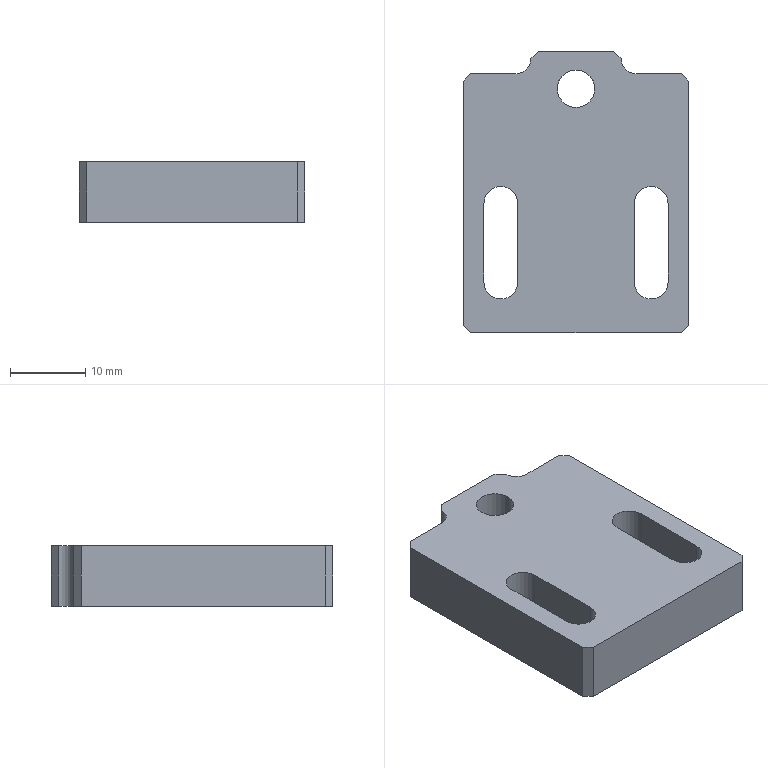Part | NX | features BREP 1 | 1 solid | 26 faces | box 30 x 37.5 x 8 mm | volume 7390 mm3 | plane 18 | cylinder 8 | commonest cylinder face diameters 4.5 x4 4 x2 5 x2
STEP:
#1=CARTESIAN_POINT('',(-6.,17.75,8.));
#2=VERTEX_POINT('',#1);
#3=CARTESIAN_POINT('',(-8.,15.75,8.));
#4=VERTEX_POINT('',#3);
#5=CARTESIAN_POINT('',(-8.,17.75,8.));
#6=DIRECTION('',(0.,0.,-1.));
#7=DIRECTION('',(-1.,0.,0.));
#8=AXIS2_PLACEMENT_3D('',#5,#6,#7);
#9=CIRCLE('',#8,2.);
#10=EDGE_CURVE('',#2,#4,#9,.T.);
#11=ORIENTED_EDGE('',*,*,#10,.F.);
#12=CARTESIAN_POINT('',(-6.,17.75,0.));
#13=VERTEX_POINT('',#12);
#14=CARTESIAN_POINT('',(-6.,17.75,8.));
#15=DIRECTION('',(0.,0.,-1.));
#16=VECTOR('',#15,1000.);
#17=LINE('',#14,#16);
#18=EDGE_CURVE('',#2,#13,#17,.T.);
#19=ORIENTED_EDGE('',*,*,#18,.T.);
#20=CARTESIAN_POINT('',(-8.,15.75,0.));
#21=VERTEX_POINT('',#20);
#22=CARTESIAN_POINT('',(-8.,17.75,0.));
#23=DIRECTION('',(0.,0.,1.));
#24=DIRECTION('',(-1.,0.,0.));
#25=AXIS2_PLACEMENT_3D('',#22,#23,#24);
#26=CIRCLE('',#25,2.);
#27=EDGE_CURVE('',#21,#13,#26,.T.);
#28=ORIENTED_EDGE('',*,*,#27,.F.);
#29=CARTESIAN_POINT('',(-8.,15.75,0.));
#30=DIRECTION('',(0.,0.,-1.));
#31=VECTOR('',#30,1000.);
#32=LINE('',#29,#31);
#33=EDGE_CURVE('',#4,#21,#32,.T.);
#34=ORIENTED_EDGE('',*,*,#33,.F.);
#35=EDGE_LOOP('',(#11,#19,#28,#34));
#36=FACE_BOUND('',#35,.T.);
#37=CARTESIAN_POINT('',(-8.,17.75,8.));
#38=DIRECTION('',(0.,0.,1.));
#39=DIRECTION('',(1.,0.,0.));
#40=AXIS2_PLACEMENT_3D('',#37,#38,#39);
#41=CYLINDRICAL_SURFACE('',#40,2.);
#42=ADVANCED_FACE('',(#36),#41,.F.);
#43=CARTESIAN_POINT('',(8.,15.75,8.));
#44=VERTEX_POINT('',#43);
#45=CARTESIAN_POINT('',(6.,17.75,8.));
#46=VERTEX_POINT('',#45);
#47=CARTESIAN_POINT('',(8.,17.75,8.));
#48=DIRECTION('',(0.,0.,-1.));
#49=DIRECTION('',(-1.,0.,0.));
#50=AXIS2_PLACEMENT_3D('',#47,#48,#49);
#51=CIRCLE('',#50,2.);
#52=EDGE_CURVE('',#44,#46,#51,.T.);
#53=ORIENTED_EDGE('',*,*,#52,.F.);
#54=CARTESIAN_POINT('',(8.,15.75,0.));
#55=VERTEX_POINT('',#54);
#56=CARTESIAN_POINT('',(8.,15.75,8.));
#57=DIRECTION('',(0.,0.,1.));
#58=VECTOR('',#57,1000.);
#59=LINE('',#56,#58);
#60=EDGE_CURVE('',#55,#44,#59,.T.);
#61=ORIENTED_EDGE('',*,*,#60,.F.);
#62=CARTESIAN_POINT('',(6.,17.75,0.));
#63=VERTEX_POINT('',#62);
#64=CARTESIAN_POINT('',(8.,17.75,0.));
#65=DIRECTION('',(0.,0.,1.));
#66=DIRECTION('',(-1.,0.,0.));
#67=AXIS2_PLACEMENT_3D('',#64,#65,#66);
#68=CIRCLE('',#67,2.);
#69=EDGE_CURVE('',#63,#55,#68,.T.);
#70=ORIENTED_EDGE('',*,*,#69,.F.);
#71=CARTESIAN_POINT('',(6.,17.75,8.));
#72=DIRECTION('',(0.,0.,1.));
#73=VECTOR('',#72,1000.);
#74=LINE('',#71,#73);
#75=EDGE_CURVE('',#63,#46,#74,.T.);
#76=ORIENTED_EDGE('',*,*,#75,.T.);
#77=EDGE_LOOP('',(#53,#61,#70,#76));
#78=FACE_BOUND('',#77,.T.);
#79=CARTESIAN_POINT('',(8.,17.75,8.));
#80=DIRECTION('',(0.,0.,1.));
#81=DIRECTION('',(1.,0.,0.));
#82=AXIS2_PLACEMENT_3D('',#79,#80,#81);
#83=CYLINDRICAL_SURFACE('',#82,2.);
#84=ADVANCED_FACE('',(#78),#83,.F.);
#85=CARTESIAN_POINT('',(-5.,18.75,8.));
#86=VERTEX_POINT('',#85);
#87=CARTESIAN_POINT('',(-6.,17.75,8.));
#88=DIRECTION('',(-0.7071,-0.7071,0.));
#89=VECTOR('',#88,1000.);
#90=LINE('',#87,#89);
#91=EDGE_CURVE('',#86,#2,#90,.T.);
#92=ORIENTED_EDGE('',*,*,#91,.F.);
#93=CARTESIAN_POINT('',(-5.,18.75,0.));
#94=VERTEX_POINT('',#93);
#95=CARTESIAN_POINT('',(-5.,18.75,8.));
#96=DIRECTION('',(0.,0.,1.));
#97=VECTOR('',#96,1000.);
#98=LINE('',#95,#97);
#99=EDGE_CURVE('',#94,#86,#98,.T.);
#100=ORIENTED_EDGE('',*,*,#99,.F.);
#101=CARTESIAN_POINT('',(-11.875,11.875,0.));
#102=DIRECTION('',(0.7071,0.7071,0.));
#103=VECTOR('',#102,1000.);
#104=LINE('',#101,#103);
#105=EDGE_CURVE('',#13,#94,#104,.T.);
#106=ORIENTED_EDGE('',*,*,#105,.F.);
#107=ORIENTED_EDGE('',*,*,#18,.F.);
#108=EDGE_LOOP('',(#92,#100,#106,#107));
#109=FACE_BOUND('',#108,.T.);
#110=CARTESIAN_POINT('',(-6.,17.75,8.));
#111=DIRECTION('',(0.7071,-0.7071,0.));
#112=DIRECTION('',(0.,0.,-1.));
#113=AXIS2_PLACEMENT_3D('',#110,#111,#112);
#114=PLANE('',#113);
#115=ADVANCED_FACE('',(#109),#114,.F.);
#116=CARTESIAN_POINT('',(-15.,-17.75,8.));
#117=VERTEX_POINT('',#116);
#118=CARTESIAN_POINT('',(-14.,-18.75,8.));
#119=VERTEX_POINT('',#118);
#120=CARTESIAN_POINT('',(-14.,-18.75,8.));
#121=DIRECTION('',(0.7071,-0.7071,0.));
#122=VECTOR('',#121,1000.);
#123=LINE('',#120,#122);
#124=EDGE_CURVE('',#117,#119,#123,.T.);
#125=ORIENTED_EDGE('',*,*,#124,.F.);
#126=CARTESIAN_POINT('',(-15.,-17.75,0.));
#127=VERTEX_POINT('',#126);
#128=CARTESIAN_POINT('',(-15.,-17.75,8.));
#129=DIRECTION('',(0.,0.,1.));
#130=VECTOR('',#129,1000.);
#131=LINE('',#128,#130);
#132=EDGE_CURVE('',#127,#117,#131,.T.);
#133=ORIENTED_EDGE('',*,*,#132,.F.);
#134=CARTESIAN_POINT('',(-14.,-18.75,0.));
#135=VERTEX_POINT('',#134);
#136=CARTESIAN_POINT('',(-16.375,-16.375,0.));
#137=DIRECTION('',(-0.7071,0.7071,0.));
#138=VECTOR('',#137,1000.);
#139=LINE('',#136,#138);
#140=EDGE_CURVE('',#135,#127,#139,.T.);
#141=ORIENTED_EDGE('',*,*,#140,.F.);
#142=CARTESIAN_POINT('',(-14.,-18.75,8.));
#143=DIRECTION('',(0.,0.,-1.));
#144=VECTOR('',#143,1000.);
#145=LINE('',#142,#144);
#146=EDGE_CURVE('',#119,#135,#145,.T.);
#147=ORIENTED_EDGE('',*,*,#146,.F.);
#148=EDGE_LOOP('',(#125,#133,#141,#147));
#149=FACE_BOUND('',#148,.T.);
#150=CARTESIAN_POINT('',(-14.,-18.75,8.));
#151=DIRECTION('',(0.7071,0.7071,0.));
#152=DIRECTION('',(0.,0.,-1.));
#153=AXIS2_PLACEMENT_3D('',#150,#151,#152);
#154=PLANE('',#153);
#155=ADVANCED_FACE('',(#149),#154,.F.);
#156=CARTESIAN_POINT('',(14.,-18.75,8.));
#157=VERTEX_POINT('',#156);
#158=CARTESIAN_POINT('',(15.,-17.75,8.));
#159=VERTEX_POINT('',#158);
#160=CARTESIAN_POINT('',(15.,-17.75,8.));
#161=DIRECTION('',(0.7071,0.7071,0.));
#162=VECTOR('',#161,1000.);
#163=LINE('',#160,#162);
#164=EDGE_CURVE('',#157,#159,#163,.T.);
#165=ORIENTED_EDGE('',*,*,#164,.F.);
#166=CARTESIAN_POINT('',(14.,-18.75,0.));
#167=VERTEX_POINT('',#166);
#168=CARTESIAN_POINT('',(14.,-18.75,8.));
#169=DIRECTION('',(0.,0.,1.));
#170=VECTOR('',#169,1000.);
#171=LINE('',#168,#170);
#172=EDGE_CURVE('',#167,#157,#171,.T.);
#173=ORIENTED_EDGE('',*,*,#172,.F.);
#174=CARTESIAN_POINT('',(15.,-17.75,0.));
#175=VERTEX_POINT('',#174);
#176=CARTESIAN_POINT('',(16.375,-16.375,0.));
#177=DIRECTION('',(-0.7071,-0.7071,0.));
#178=VECTOR('',#177,1000.);
#179=LINE('',#176,#178);
#180=EDGE_CURVE('',#175,#167,#179,.T.);
#181=ORIENTED_EDGE('',*,*,#180,.F.);
#182=CARTESIAN_POINT('',(15.,-17.75,8.));
#183=DIRECTION('',(0.,0.,-1.));
#184=VECTOR('',#183,1000.);
#185=LINE('',#182,#184);
#186=EDGE_CURVE('',#159,#175,#185,.T.);
#187=ORIENTED_EDGE('',*,*,#186,.F.);
#188=EDGE_LOOP('',(#165,#173,#181,#187));
#189=FACE_BOUND('',#188,.T.);
#190=CARTESIAN_POINT('',(15.,-17.75,8.));
#191=DIRECTION('',(-0.7071,0.7071,0.));
#192=DIRECTION('',(0.,0.,-1.));
#193=AXIS2_PLACEMENT_3D('',#190,#191,#192);
#194=PLANE('',#193);
#195=ADVANCED_FACE('',(#189),#194,.F.);
#196=CARTESIAN_POINT('',(-14.,15.75,8.));
#197=VERTEX_POINT('',#196);
#198=CARTESIAN_POINT('',(-15.,14.75,8.));
#199=VERTEX_POINT('',#198);
#200=CARTESIAN_POINT('',(-15.,14.75,8.));
#201=DIRECTION('',(-0.7071,-0.7071,0.));
#202=VECTOR('',#201,1000.);
#203=LINE('',#200,#202);
#204=EDGE_CURVE('',#197,#199,#203,.T.);
#205=ORIENTED_EDGE('',*,*,#204,.F.);
#206=CARTESIAN_POINT('',(-14.,15.75,0.));
#207=VERTEX_POINT('',#206);
#208=CARTESIAN_POINT('',(-14.,15.75,8.));
#209=DIRECTION('',(0.,0.,1.));
#210=VECTOR('',#209,1000.);
#211=LINE('',#208,#210);
#212=EDGE_CURVE('',#207,#197,#211,.T.);
#213=ORIENTED_EDGE('',*,*,#212,.F.);
#214=CARTESIAN_POINT('',(-15.,14.75,0.));
#215=VERTEX_POINT('',#214);
#216=CARTESIAN_POINT('',(-14.875,14.875,0.));
#217=DIRECTION('',(0.7071,0.7071,0.));
#218=VECTOR('',#217,1000.);
#219=LINE('',#216,#218);
#220=EDGE_CURVE('',#215,#207,#219,.T.);
#221=ORIENTED_EDGE('',*,*,#220,.F.);
#222=CARTESIAN_POINT('',(-15.,14.75,8.));
#223=DIRECTION('',(0.,0.,-1.));
#224=VECTOR('',#223,1000.);
#225=LINE('',#222,#224);
#226=EDGE_CURVE('',#199,#215,#225,.T.);
#227=ORIENTED_EDGE('',*,*,#226,.F.);
#228=EDGE_LOOP('',(#205,#213,#221,#227));
#229=FACE_BOUND('',#228,.T.);
#230=CARTESIAN_POINT('',(-15.,14.75,8.));
#231=DIRECTION('',(0.7071,-0.7071,0.));
#232=DIRECTION('',(0.,0.,-1.));
#233=AXIS2_PLACEMENT_3D('',#230,#231,#232);
#234=PLANE('',#233);
#235=ADVANCED_FACE('',(#229),#234,.F.);
#236=CARTESIAN_POINT('',(15.,14.75,8.));
#237=VERTEX_POINT('',#236);
#238=CARTESIAN_POINT('',(14.,15.75,8.));
#239=VERTEX_POINT('',#238);
#240=CARTESIAN_POINT('',(14.,15.75,8.));
#241=DIRECTION('',(-0.7071,0.7071,0.));
#242=VECTOR('',#241,1000.);
#243=LINE('',#240,#242);
#244=EDGE_CURVE('',#237,#239,#243,.T.);
#245=ORIENTED_EDGE('',*,*,#244,.F.);
#246=CARTESIAN_POINT('',(15.,14.75,0.));
#247=VERTEX_POINT('',#246);
#248=CARTESIAN_POINT('',(15.,14.75,8.));
#249=DIRECTION('',(0.,0.,1.));
#250=VECTOR('',#249,1000.);
#251=LINE('',#248,#250);
#252=EDGE_CURVE('',#247,#237,#251,.T.);
#253=ORIENTED_EDGE('',*,*,#252,.F.);
#254=CARTESIAN_POINT('',(14.,15.75,0.));
#255=VERTEX_POINT('',#254);
#256=CARTESIAN_POINT('',(14.875,14.875,0.));
#257=DIRECTION('',(0.7071,-0.7071,0.));
#258=VECTOR('',#257,1000.);
#259=LINE('',#256,#258);
#260=EDGE_CURVE('',#255,#247,#259,.T.);
#261=ORIENTED_EDGE('',*,*,#260,.F.);
#262=CARTESIAN_POINT('',(14.,15.75,8.));
#263=DIRECTION('',(0.,0.,-1.));
#264=VECTOR('',#263,1000.);
#265=LINE('',#262,#264);
#266=EDGE_CURVE('',#239,#255,#265,.T.);
#267=ORIENTED_EDGE('',*,*,#266,.F.);
#268=EDGE_LOOP('',(#245,#253,#261,#267));
#269=FACE_BOUND('',#268,.T.);
#270=CARTESIAN_POINT('',(14.,15.75,8.));
#271=DIRECTION('',(-0.7071,-0.7071,0.));
#272=DIRECTION('',(0.,0.,-1.));
#273=AXIS2_PLACEMENT_3D('',#270,#271,#272);
#274=PLANE('',#273);
#275=ADVANCED_FACE('',(#269),#274,.F.);
#276=CARTESIAN_POINT('',(5.,18.75,8.));
#277=VERTEX_POINT('',#276);
#278=CARTESIAN_POINT('',(5.,18.75,8.));
#279=DIRECTION('',(-0.7071,0.7071,0.));
#280=VECTOR('',#279,1000.);
#281=LINE('',#278,#280);
#282=EDGE_CURVE('',#46,#277,#281,.T.);
#283=ORIENTED_EDGE('',*,*,#282,.F.);
#284=ORIENTED_EDGE('',*,*,#75,.F.);
#285=CARTESIAN_POINT('',(5.,18.75,0.));
#286=VERTEX_POINT('',#285);
#287=CARTESIAN_POINT('',(11.875,11.875,0.));
#288=DIRECTION('',(0.7071,-0.7071,0.));
#289=VECTOR('',#288,1000.);
#290=LINE('',#287,#289);
#291=EDGE_CURVE('',#286,#63,#290,.T.);
#292=ORIENTED_EDGE('',*,*,#291,.F.);
#293=CARTESIAN_POINT('',(5.,18.75,8.));
#294=DIRECTION('',(0.,0.,-1.));
#295=VECTOR('',#294,1000.);
#296=LINE('',#293,#295);
#297=EDGE_CURVE('',#277,#286,#296,.T.);
#298=ORIENTED_EDGE('',*,*,#297,.F.);
#299=EDGE_LOOP('',(#283,#284,#292,#298));
#300=FACE_BOUND('',#299,.T.);
#301=CARTESIAN_POINT('',(5.,18.75,8.));
#302=DIRECTION('',(-0.7071,-0.7071,0.));
#303=DIRECTION('',(0.,0.,-1.));
#304=AXIS2_PLACEMENT_3D('',#301,#302,#303);
#305=PLANE('',#304);
#306=ADVANCED_FACE('',(#300),#305,.F.);
#307=CARTESIAN_POINT('',(-12.25,-1.5,0.));
#308=VERTEX_POINT('',#307);
#309=CARTESIAN_POINT('',(-12.25,-1.5,8.));
#310=VERTEX_POINT('',#309);
#311=CARTESIAN_POINT('',(-12.25,-1.5,0.));
#312=DIRECTION('',(0.,0.,1.));
#313=VECTOR('',#312,1000.);
#314=LINE('',#311,#313);
#315=EDGE_CURVE('',#308,#310,#314,.T.);
#316=ORIENTED_EDGE('',*,*,#315,.T.);
#317=CARTESIAN_POINT('',(-12.25,-12.,8.));
#318=VERTEX_POINT('',#317);
#319=CARTESIAN_POINT('',(-12.25,-12.,8.));
#320=DIRECTION('',(0.,1.,0.));
#321=VECTOR('',#320,1000.);
#322=LINE('',#319,#321);
#323=EDGE_CURVE('',#318,#310,#322,.T.);
#324=ORIENTED_EDGE('',*,*,#323,.F.);
#325=CARTESIAN_POINT('',(-12.25,-12.,0.));
#326=VERTEX_POINT('',#325);
#327=CARTESIAN_POINT('',(-12.25,-12.,0.));
#328=DIRECTION('',(0.,0.,-1.));
#329=VECTOR('',#328,1000.);
#330=LINE('',#327,#329);
#331=EDGE_CURVE('',#318,#326,#330,.T.);
#332=ORIENTED_EDGE('',*,*,#331,.T.);
#333=CARTESIAN_POINT('',(-12.25,-12.,0.));
#334=DIRECTION('',(0.,1.,0.));
#335=VECTOR('',#334,1000.);
#336=LINE('',#333,#335);
#337=EDGE_CURVE('',#326,#308,#336,.T.);
#338=ORIENTED_EDGE('',*,*,#337,.T.);
#339=EDGE_LOOP('',(#316,#324,#332,#338));
#340=FACE_BOUND('',#339,.T.);
#341=CARTESIAN_POINT('',(-12.25,-12.,0.));
#342=DIRECTION('',(-1.,0.,0.));
#343=DIRECTION('',(0.,0.,1.));
#344=AXIS2_PLACEMENT_3D('',#341,#342,#343);
#345=PLANE('',#344);
#346=ADVANCED_FACE('',(#340),#345,.F.);
#347=CARTESIAN_POINT('',(-7.75,-1.5,0.));
#348=VERTEX_POINT('',#347);
#349=CARTESIAN_POINT('',(-7.75,-1.5,8.));
#350=VERTEX_POINT('',#349);
#351=CARTESIAN_POINT('',(-7.75,-1.5,8.));
#352=DIRECTION('',(0.,0.,1.));
#353=VECTOR('',#352,1000.);
#354=LINE('',#351,#353);
#355=EDGE_CURVE('',#348,#350,#354,.T.);
#356=ORIENTED_EDGE('',*,*,#355,.F.);
#357=CARTESIAN_POINT('',(-7.75,-12.,0.));
#358=VERTEX_POINT('',#357);
#359=CARTESIAN_POINT('',(-7.75,-12.,0.));
#360=DIRECTION('',(0.,1.,0.));
#361=VECTOR('',#360,1000.);
#362=LINE('',#359,#361);
#363=EDGE_CURVE('',#358,#348,#362,.T.);
#364=ORIENTED_EDGE('',*,*,#363,.F.);
#365=CARTESIAN_POINT('',(-7.75,-12.,8.));
#366=VERTEX_POINT('',#365);
#367=CARTESIAN_POINT('',(-7.75,-12.,8.));
#368=DIRECTION('',(0.,0.,1.));
#369=VECTOR('',#368,1000.);
#370=LINE('',#367,#369);
#371=EDGE_CURVE('',#358,#366,#370,.T.);
#372=ORIENTED_EDGE('',*,*,#371,.T.);
#373=CARTESIAN_POINT('',(-7.75,-12.,8.));
#374=DIRECTION('',(0.,1.,0.));
#375=VECTOR('',#374,1000.);
#376=LINE('',#373,#375);
#377=EDGE_CURVE('',#366,#350,#376,.T.);
#378=ORIENTED_EDGE('',*,*,#377,.T.);
#379=EDGE_LOOP('',(#356,#364,#372,#378));
#380=FACE_BOUND('',#379,.T.);
#381=CARTESIAN_POINT('',(-7.75,-12.,8.));
#382=DIRECTION('',(-1.,0.,0.));
#383=DIRECTION('',(0.,0.,1.));
#384=AXIS2_PLACEMENT_3D('',#381,#382,#383);
#385=PLANE('',#384);
#386=ADVANCED_FACE('',(#380),#385,.T.);
#387=CARTESIAN_POINT('',(-10.,-12.,8.));
#388=DIRECTION('',(0.,0.,-1.));
#389=DIRECTION('',(-1.,0.,0.));
#390=AXIS2_PLACEMENT_3D('',#387,#388,#389);
#391=CIRCLE('',#390,2.25);
#392=EDGE_CURVE('',#366,#318,#391,.T.);
#393=ORIENTED_EDGE('',*,*,#392,.F.);
#394=ORIENTED_EDGE('',*,*,#371,.F.);
#395=CARTESIAN_POINT('',(-10.,-12.,0.));
#396=DIRECTION('',(0.,0.,-1.));
#397=DIRECTION('',(-1.,0.,0.));
#398=AXIS2_PLACEMENT_3D('',#395,#396,#397);
#399=CIRCLE('',#398,2.25);
#400=EDGE_CURVE('',#358,#326,#399,.T.);
#401=ORIENTED_EDGE('',*,*,#400,.T.);
#402=ORIENTED_EDGE('',*,*,#331,.F.);
#403=EDGE_LOOP('',(#393,#394,#401,#402));
#404=FACE_BOUND('',#403,.T.);
#405=CARTESIAN_POINT('',(-10.,-12.,0.));
#406=DIRECTION('',(0.,0.,-1.));
#407=DIRECTION('',(-1.,0.,0.));
#408=AXIS2_PLACEMENT_3D('',#405,#406,#407);
#409=CYLINDRICAL_SURFACE('',#408,2.25);
#410=ADVANCED_FACE('',(#404),#409,.F.);
#411=CARTESIAN_POINT('',(-10.,-1.5,0.));
#412=DIRECTION('',(0.,0.,-1.));
#413=DIRECTION('',(-1.,0.,0.));
#414=AXIS2_PLACEMENT_3D('',#411,#412,#413);
#415=CIRCLE('',#414,2.25);
#416=EDGE_CURVE('',#308,#348,#415,.T.);
#417=ORIENTED_EDGE('',*,*,#416,.T.);
#418=ORIENTED_EDGE('',*,*,#355,.T.);
#419=CARTESIAN_POINT('',(-10.,-1.5,8.));
#420=DIRECTION('',(0.,0.,-1.));
#421=DIRECTION('',(-1.,0.,0.));
#422=AXIS2_PLACEMENT_3D('',#419,#420,#421);
#423=CIRCLE('',#422,2.25);
#424=EDGE_CURVE('',#310,#350,#423,.T.);
#425=ORIENTED_EDGE('',*,*,#424,.F.);
#426=ORIENTED_EDGE('',*,*,#315,.F.);
#427=EDGE_LOOP('',(#417,#418,#425,#426));
#428=FACE_BOUND('',#427,.T.);
#429=CARTESIAN_POINT('',(-10.,-1.5,0.));
#430=DIRECTION('',(0.,0.,-1.));
#431=DIRECTION('',(-1.,0.,0.));
#432=AXIS2_PLACEMENT_3D('',#429,#430,#431);
#433=CYLINDRICAL_SURFACE('',#432,2.25);
#434=ADVANCED_FACE('',(#428),#433,.F.);
#435=CARTESIAN_POINT('',(7.75,-1.5,0.));
#436=VERTEX_POINT('',#435);
#437=CARTESIAN_POINT('',(7.75,-1.5,8.));
#438=VERTEX_POINT('',#437);
#439=CARTESIAN_POINT('',(7.75,-1.5,0.));
#440=DIRECTION('',(0.,0.,1.));
#441=VECTOR('',#440,1000.);
#442=LINE('',#439,#441);
#443=EDGE_CURVE('',#436,#438,#442,.T.);
#444=ORIENTED_EDGE('',*,*,#443,.T.);
#445=CARTESIAN_POINT('',(7.75,-12.,8.));
#446=VERTEX_POINT('',#445);
#447=CARTESIAN_POINT('',(7.75,-12.,8.));
#448=DIRECTION('',(0.,1.,0.));
#449=VECTOR('',#448,1000.);
#450=LINE('',#447,#449);
#451=EDGE_CURVE('',#446,#438,#450,.T.);
#452=ORIENTED_EDGE('',*,*,#451,.F.);
#453=CARTESIAN_POINT('',(7.75,-12.,0.));
#454=VERTEX_POINT('',#453);
#455=CARTESIAN_POINT('',(7.75,-12.,0.));
#456=DIRECTION('',(0.,0.,-1.));
#457=VECTOR('',#456,1000.);
#458=LINE('',#455,#457);
#459=EDGE_CURVE('',#446,#454,#458,.T.);
#460=ORIENTED_EDGE('',*,*,#459,.T.);
#461=CARTESIAN_POINT('',(7.75,-12.,0.));
#462=DIRECTION('',(0.,1.,0.));
#463=VECTOR('',#462,1000.);
#464=LINE('',#461,#463);
#465=EDGE_CURVE('',#454,#436,#464,.T.);
#466=ORIENTED_EDGE('',*,*,#465,.T.);
#467=EDGE_LOOP('',(#444,#452,#460,#466));
#468=FACE_BOUND('',#467,.T.);
#469=CARTESIAN_POINT('',(7.75,-12.,0.));
#470=DIRECTION('',(-1.,0.,0.));
#471=DIRECTION('',(0.,0.,1.));
#472=AXIS2_PLACEMENT_3D('',#469,#470,#471);
#473=PLANE('',#472);
#474=ADVANCED_FACE('',(#468),#473,.F.);
#475=CARTESIAN_POINT('',(12.25,-1.5,0.));
#476=VERTEX_POINT('',#475);
#477=CARTESIAN_POINT('',(12.25,-1.5,8.));
#478=VERTEX_POINT('',#477);
#479=CARTESIAN_POINT('',(12.25,-1.5,8.));
#480=DIRECTION('',(0.,0.,1.));
#481=VECTOR('',#480,1000.);
#482=LINE('',#479,#481);
#483=EDGE_CURVE('',#476,#478,#482,.T.);
#484=ORIENTED_EDGE('',*,*,#483,.F.);
#485=CARTESIAN_POINT('',(12.25,-12.,0.));
#486=VERTEX_POINT('',#485);
#487=CARTESIAN_POINT('',(12.25,-12.,0.));
#488=DIRECTION('',(0.,1.,0.));
#489=VECTOR('',#488,1000.);
#490=LINE('',#487,#489);
#491=EDGE_CURVE('',#486,#476,#490,.T.);
#492=ORIENTED_EDGE('',*,*,#491,.F.);
#493=CARTESIAN_POINT('',(12.25,-12.,8.));
#494=VERTEX_POINT('',#493);
#495=CARTESIAN_POINT('',(12.25,-12.,8.));
#496=DIRECTION('',(0.,0.,1.));
#497=VECTOR('',#496,1000.);
#498=LINE('',#495,#497);
#499=EDGE_CURVE('',#486,#494,#498,.T.);
#500=ORIENTED_EDGE('',*,*,#499,.T.);
#501=CARTESIAN_POINT('',(12.25,-12.,8.));
#502=DIRECTION('',(0.,1.,0.));
#503=VECTOR('',#502,1000.);
#504=LINE('',#501,#503);
#505=EDGE_CURVE('',#494,#478,#504,.T.);
#506=ORIENTED_EDGE('',*,*,#505,.T.);
#507=EDGE_LOOP('',(#484,#492,#500,#506));
#508=FACE_BOUND('',#507,.T.);
#509=CARTESIAN_POINT('',(12.25,-12.,8.));
#510=DIRECTION('',(-1.,0.,0.));
#511=DIRECTION('',(0.,0.,1.));
#512=AXIS2_PLACEMENT_3D('',#509,#510,#511);
#513=PLANE('',#512);
#514=ADVANCED_FACE('',(#508),#513,.T.);
#515=CARTESIAN_POINT('',(10.,-12.,8.));
#516=DIRECTION('',(0.,0.,-1.));
#517=DIRECTION('',(-1.,0.,0.));
#518=AXIS2_PLACEMENT_3D('',#515,#516,#517);
#519=CIRCLE('',#518,2.25);
#520=EDGE_CURVE('',#494,#446,#519,.T.);
#521=ORIENTED_EDGE('',*,*,#520,.F.);
#522=ORIENTED_EDGE('',*,*,#499,.F.);
#523=CARTESIAN_POINT('',(10.,-12.,0.));
#524=DIRECTION('',(0.,0.,-1.));
#525=DIRECTION('',(-1.,0.,0.));
#526=AXIS2_PLACEMENT_3D('',#523,#524,#525);
#527=CIRCLE('',#526,2.25);
#528=EDGE_CURVE('',#486,#454,#527,.T.);
#529=ORIENTED_EDGE('',*,*,#528,.T.);
#530=ORIENTED_EDGE('',*,*,#459,.F.);
#531=EDGE_LOOP('',(#521,#522,#529,#530));
#532=FACE_BOUND('',#531,.T.);
#533=CARTESIAN_POINT('',(10.,-12.,0.));
#534=DIRECTION('',(0.,0.,-1.));
#535=DIRECTION('',(-1.,0.,0.));
#536=AXIS2_PLACEMENT_3D('',#533,#534,#535);
#537=CYLINDRICAL_SURFACE('',#536,2.25);
#538=ADVANCED_FACE('',(#532),#537,.F.);
#539=CARTESIAN_POINT('',(10.,-1.5,0.));
#540=DIRECTION('',(0.,0.,-1.));
#541=DIRECTION('',(-1.,0.,0.));
#542=AXIS2_PLACEMENT_3D('',#539,#540,#541);
#543=CIRCLE('',#542,2.25);
#544=EDGE_CURVE('',#436,#476,#543,.T.);
#545=ORIENTED_EDGE('',*,*,#544,.T.);
#546=ORIENTED_EDGE('',*,*,#483,.T.);
#547=CARTESIAN_POINT('',(10.,-1.5,8.));
#548=DIRECTION('',(0.,0.,-1.));
#549=DIRECTION('',(-1.,0.,0.));
#550=AXIS2_PLACEMENT_3D('',#547,#548,#549);
#551=CIRCLE('',#550,2.25);
#552=EDGE_CURVE('',#438,#478,#551,.T.);
#553=ORIENTED_EDGE('',*,*,#552,.F.);
#554=ORIENTED_EDGE('',*,*,#443,.F.);
#555=EDGE_LOOP('',(#545,#546,#553,#554));
#556=FACE_BOUND('',#555,.T.);
#557=CARTESIAN_POINT('',(10.,-1.5,0.));
#558=DIRECTION('',(0.,0.,-1.));
#559=DIRECTION('',(-1.,0.,0.));
#560=AXIS2_PLACEMENT_3D('',#557,#558,#559);
#561=CYLINDRICAL_SURFACE('',#560,2.25);
#562=ADVANCED_FACE('',(#556),#561,.F.);
#563=CARTESIAN_POINT('',(-15.,15.75,8.));
#564=DIRECTION('',(-1.,0.,0.));
#565=VECTOR('',#564,1000.);
#566=LINE('',#563,#565);
#567=EDGE_CURVE('',#4,#197,#566,.T.);
#568=ORIENTED_EDGE('',*,*,#567,.F.);
#569=ORIENTED_EDGE('',*,*,#33,.T.);
#570=CARTESIAN_POINT('',(-15.,15.75,0.));
#571=DIRECTION('',(-1.,0.,0.));
#572=VECTOR('',#571,1000.);
#573=LINE('',#570,#572);
#574=EDGE_CURVE('',#21,#207,#573,.T.);
#575=ORIENTED_EDGE('',*,*,#574,.T.);
#576=ORIENTED_EDGE('',*,*,#212,.T.);
#577=EDGE_LOOP('',(#568,#569,#575,#576));
#578=FACE_BOUND('',#577,.T.);
#579=CARTESIAN_POINT('',(-15.,15.75,8.));
#580=DIRECTION('',(0.,-1.,0.));
#581=DIRECTION('',(0.,0.,-1.));
#582=AXIS2_PLACEMENT_3D('',#579,#580,#581);
#583=PLANE('',#582);
#584=ADVANCED_FACE('',(#578),#583,.F.);
#585=CARTESIAN_POINT('',(15.,15.75,0.));
#586=DIRECTION('',(-1.,0.,0.));
#587=VECTOR('',#586,1000.);
#588=LINE('',#585,#587);
#589=EDGE_CURVE('',#255,#55,#588,.T.);
#590=ORIENTED_EDGE('',*,*,#589,.T.);
#591=ORIENTED_EDGE('',*,*,#60,.T.);
#592=CARTESIAN_POINT('',(15.,15.75,8.));
#593=DIRECTION('',(-1.,0.,0.));
#594=VECTOR('',#593,1000.);
#595=LINE('',#592,#594);
#596=EDGE_CURVE('',#239,#44,#595,.T.);
#597=ORIENTED_EDGE('',*,*,#596,.F.);
#598=ORIENTED_EDGE('',*,*,#266,.T.);
#599=EDGE_LOOP('',(#590,#591,#597,#598));
#600=FACE_BOUND('',#599,.T.);
#601=CARTESIAN_POINT('',(15.,15.75,8.));
#602=DIRECTION('',(0.,-1.,0.));
#603=DIRECTION('',(1.,0.,0.));
#604=AXIS2_PLACEMENT_3D('',#601,#602,#603);
#605=PLANE('',#604);
#606=ADVANCED_FACE('',(#600),#605,.F.);
#607=CARTESIAN_POINT('',(-2.5,13.75,8.));
#608=VERTEX_POINT('',#607);
#609=CARTESIAN_POINT('',(-2.5,13.75,0.));
#610=VERTEX_POINT('',#609);
#611=CARTESIAN_POINT('',(-2.5,13.75,8.));
#612=DIRECTION('',(0.,0.,1.));
#613=VECTOR('',#612,1000.);
#614=LINE('',#611,#613);
#615=EDGE_CURVE('',#608,#610,#614,.F.);
#616=ORIENTED_EDGE('',*,*,#615,.T.);
#617=CARTESIAN_POINT('',(2.5,13.75,0.));
#618=VERTEX_POINT('',#617);
#619=CARTESIAN_POINT('',(0.,13.75,0.));
#620=DIRECTION('',(0.,0.,1.));
#621=DIRECTION('',(1.,0.,0.));
#622=AXIS2_PLACEMENT_3D('',#619,#620,#621);
#623=CIRCLE('',#622,2.5);
#624=EDGE_CURVE('',#618,#610,#623,.T.);
#625=ORIENTED_EDGE('',*,*,#624,.F.);
#626=CARTESIAN_POINT('',(2.5,13.75,8.));
#627=VERTEX_POINT('',#626);
#628=CARTESIAN_POINT('',(2.5,13.75,8.));
#629=DIRECTION('',(0.,0.,1.));
#630=VECTOR('',#629,1000.);
#631=LINE('',#628,#630);
#632=EDGE_CURVE('',#627,#618,#631,.F.);
#633=ORIENTED_EDGE('',*,*,#632,.F.);
#634=CARTESIAN_POINT('',(0.,13.75,8.));
#635=DIRECTION('',(0.,0.,1.));
#636=DIRECTION('',(1.,0.,0.));
#637=AXIS2_PLACEMENT_3D('',#634,#635,#636);
#638=CIRCLE('',#637,2.5);
#639=EDGE_CURVE('',#627,#608,#638,.T.);
#640=ORIENTED_EDGE('',*,*,#639,.T.);
#641=EDGE_LOOP('',(#616,#625,#633,#640));
#642=FACE_BOUND('',#641,.T.);
#643=CARTESIAN_POINT('',(0.,13.75,8.));
#644=DIRECTION('',(0.,0.,1.));
#645=DIRECTION('',(1.,0.,0.));
#646=AXIS2_PLACEMENT_3D('',#643,#644,#645);
#647=CYLINDRICAL_SURFACE('',#646,2.5);
#648=ADVANCED_FACE('',(#642),#647,.F.);
#649=ORIENTED_EDGE('',*,*,#624,.T.);
#650=CARTESIAN_POINT('',(0.,13.75,0.));
#651=DIRECTION('',(0.,0.,1.));
#652=DIRECTION('',(1.,0.,0.));
#653=AXIS2_PLACEMENT_3D('',#650,#651,#652);
#654=CIRCLE('',#653,2.5);
#655=EDGE_CURVE('',#610,#618,#654,.T.);
#656=ORIENTED_EDGE('',*,*,#655,.T.);
#657=EDGE_LOOP('',(#649,#656));
#658=FACE_BOUND('',#657,.T.);
#659=CARTESIAN_POINT('',(-15.,18.75,0.));
#660=DIRECTION('',(-1.,0.,0.));
#661=VECTOR('',#660,1000.);
#662=LINE('',#659,#661);
#663=EDGE_CURVE('',#286,#94,#662,.T.);
#664=ORIENTED_EDGE('',*,*,#663,.F.);
#665=ORIENTED_EDGE('',*,*,#291,.T.);
#666=ORIENTED_EDGE('',*,*,#69,.T.);
#667=ORIENTED_EDGE('',*,*,#589,.F.);
#668=ORIENTED_EDGE('',*,*,#260,.T.);
#669=CARTESIAN_POINT('',(15.,-18.75,0.));
#670=DIRECTION('',(0.,1.,0.));
#671=VECTOR('',#670,1000.);
#672=LINE('',#669,#671);
#673=EDGE_CURVE('',#175,#247,#672,.T.);
#674=ORIENTED_EDGE('',*,*,#673,.F.);
#675=ORIENTED_EDGE('',*,*,#180,.T.);
#676=CARTESIAN_POINT('',(-15.,-18.75,0.));
#677=DIRECTION('',(1.,0.,0.));
#678=VECTOR('',#677,1000.);
#679=LINE('',#676,#678);
#680=EDGE_CURVE('',#135,#167,#679,.T.);
#681=ORIENTED_EDGE('',*,*,#680,.F.);
#682=ORIENTED_EDGE('',*,*,#140,.T.);
#683=CARTESIAN_POINT('',(-15.,-18.75,0.));
#684=DIRECTION('',(0.,-1.,0.));
#685=VECTOR('',#684,1000.);
#686=LINE('',#683,#685);
#687=EDGE_CURVE('',#215,#127,#686,.T.);
#688=ORIENTED_EDGE('',*,*,#687,.F.);
#689=ORIENTED_EDGE('',*,*,#220,.T.);
#690=ORIENTED_EDGE('',*,*,#574,.F.);
#691=ORIENTED_EDGE('',*,*,#27,.T.);
#692=ORIENTED_EDGE('',*,*,#105,.T.);
#693=EDGE_LOOP('',(#664,#665,#666,#667,#668,#674,#675,#681,#682,#688,#689,#690,#691,#692));
#694=FACE_BOUND('',#693,.T.);
#695=ORIENTED_EDGE('',*,*,#465,.F.);
#696=ORIENTED_EDGE('',*,*,#528,.F.);
#697=ORIENTED_EDGE('',*,*,#491,.T.);
#698=ORIENTED_EDGE('',*,*,#544,.F.);
#699=EDGE_LOOP('',(#695,#696,#697,#698));
#700=FACE_BOUND('',#699,.T.);
#701=ORIENTED_EDGE('',*,*,#337,.F.);
#702=ORIENTED_EDGE('',*,*,#400,.F.);
#703=ORIENTED_EDGE('',*,*,#363,.T.);
#704=ORIENTED_EDGE('',*,*,#416,.F.);
#705=EDGE_LOOP('',(#701,#702,#703,#704));
#706=FACE_BOUND('',#705,.T.);
#707=CARTESIAN_POINT('',(0.,0.,0.));
#708=DIRECTION('',(0.,0.,-1.));
#709=DIRECTION('',(-1.,0.,0.));
#710=AXIS2_PLACEMENT_3D('',#707,#708,#709);
#711=PLANE('',#710);
#712=ADVANCED_FACE('',(#658,#694,#700,#706),#711,.T.);
#713=ORIENTED_EDGE('',*,*,#596,.T.);
#714=ORIENTED_EDGE('',*,*,#52,.T.);
#715=ORIENTED_EDGE('',*,*,#282,.T.);
#716=CARTESIAN_POINT('',(-15.,18.75,8.));
#717=DIRECTION('',(-1.,0.,0.));
#718=VECTOR('',#717,1000.);
#719=LINE('',#716,#718);
#720=EDGE_CURVE('',#277,#86,#719,.T.);
#721=ORIENTED_EDGE('',*,*,#720,.T.);
#722=ORIENTED_EDGE('',*,*,#91,.T.);
#723=ORIENTED_EDGE('',*,*,#10,.T.);
#724=ORIENTED_EDGE('',*,*,#567,.T.);
#725=ORIENTED_EDGE('',*,*,#204,.T.);
#726=CARTESIAN_POINT('',(-15.,-18.75,8.));
#727=DIRECTION('',(0.,-1.,0.));
#728=VECTOR('',#727,1000.);
#729=LINE('',#726,#728);
#730=EDGE_CURVE('',#199,#117,#729,.T.);
#731=ORIENTED_EDGE('',*,*,#730,.T.);
#732=ORIENTED_EDGE('',*,*,#124,.T.);
#733=CARTESIAN_POINT('',(-15.,-18.75,8.));
#734=DIRECTION('',(1.,0.,0.));
#735=VECTOR('',#734,1000.);
#736=LINE('',#733,#735);
#737=EDGE_CURVE('',#119,#157,#736,.T.);
#738=ORIENTED_EDGE('',*,*,#737,.T.);
#739=ORIENTED_EDGE('',*,*,#164,.T.);
#740=CARTESIAN_POINT('',(15.,-18.75,8.));
#741=DIRECTION('',(0.,1.,0.));
#742=VECTOR('',#741,1000.);
#743=LINE('',#740,#742);
#744=EDGE_CURVE('',#159,#237,#743,.T.);
#745=ORIENTED_EDGE('',*,*,#744,.T.);
#746=ORIENTED_EDGE('',*,*,#244,.T.);
#747=EDGE_LOOP('',(#713,#714,#715,#721,#722,#723,#724,#725,#731,#732,#738,#739,#745,#746));
#748=FACE_BOUND('',#747,.T.);
#749=ORIENTED_EDGE('',*,*,#639,.F.);
#750=CARTESIAN_POINT('',(0.,13.75,8.));
#751=DIRECTION('',(0.,0.,1.));
#752=DIRECTION('',(1.,0.,0.));
#753=AXIS2_PLACEMENT_3D('',#750,#751,#752);
#754=CIRCLE('',#753,2.5);
#755=EDGE_CURVE('',#608,#627,#754,.T.);
#756=ORIENTED_EDGE('',*,*,#755,.F.);
#757=EDGE_LOOP('',(#749,#756));
#758=FACE_BOUND('',#757,.T.);
#759=ORIENTED_EDGE('',*,*,#451,.T.);
#760=ORIENTED_EDGE('',*,*,#552,.T.);
#761=ORIENTED_EDGE('',*,*,#505,.F.);
#762=ORIENTED_EDGE('',*,*,#520,.T.);
#763=EDGE_LOOP('',(#759,#760,#761,#762));
#764=FACE_BOUND('',#763,.T.);
#765=ORIENTED_EDGE('',*,*,#323,.T.);
#766=ORIENTED_EDGE('',*,*,#424,.T.);
#767=ORIENTED_EDGE('',*,*,#377,.F.);
#768=ORIENTED_EDGE('',*,*,#392,.T.);
#769=EDGE_LOOP('',(#765,#766,#767,#768));
#770=FACE_BOUND('',#769,.T.);
#771=CARTESIAN_POINT('',(0.,0.,8.));
#772=DIRECTION('',(0.,0.,-1.));
#773=DIRECTION('',(-1.,0.,0.));
#774=AXIS2_PLACEMENT_3D('',#771,#772,#773);
#775=PLANE('',#774);
#776=ADVANCED_FACE('',(#748,#758,#764,#770),#775,.F.);
#777=ORIENTED_EDGE('',*,*,#680,.T.);
#778=ORIENTED_EDGE('',*,*,#172,.T.);
#779=ORIENTED_EDGE('',*,*,#737,.F.);
#780=ORIENTED_EDGE('',*,*,#146,.T.);
#781=EDGE_LOOP('',(#777,#778,#779,#780));
#782=FACE_BOUND('',#781,.T.);
#783=CARTESIAN_POINT('',(-15.,-18.75,8.));
#784=DIRECTION('',(0.,1.,0.));
#785=DIRECTION('',(0.,0.,1.));
#786=AXIS2_PLACEMENT_3D('',#783,#784,#785);
#787=PLANE('',#786);
#788=ADVANCED_FACE('',(#782),#787,.F.);
#789=ORIENTED_EDGE('',*,*,#730,.F.);
#790=ORIENTED_EDGE('',*,*,#226,.T.);
#791=ORIENTED_EDGE('',*,*,#687,.T.);
#792=ORIENTED_EDGE('',*,*,#132,.T.);
#793=EDGE_LOOP('',(#789,#790,#791,#792));
#794=FACE_BOUND('',#793,.T.);
#795=CARTESIAN_POINT('',(-15.,-18.75,8.));
#796=DIRECTION('',(1.,0.,0.));
#797=DIRECTION('',(0.,0.,-1.));
#798=AXIS2_PLACEMENT_3D('',#795,#796,#797);
#799=PLANE('',#798);
#800=ADVANCED_FACE('',(#794),#799,.F.);
#801=ORIENTED_EDGE('',*,*,#720,.F.);
#802=ORIENTED_EDGE('',*,*,#297,.T.);
#803=ORIENTED_EDGE('',*,*,#663,.T.);
#804=ORIENTED_EDGE('',*,*,#99,.T.);
#805=EDGE_LOOP('',(#801,#802,#803,#804));
#806=FACE_BOUND('',#805,.T.);
#807=CARTESIAN_POINT('',(-15.,18.75,8.));
#808=DIRECTION('',(0.,-1.,0.));
#809=DIRECTION('',(0.,0.,-1.));
#810=AXIS2_PLACEMENT_3D('',#807,#808,#809);
#811=PLANE('',#810);
#812=ADVANCED_FACE('',(#806),#811,.F.);
#813=ORIENTED_EDGE('',*,*,#673,.T.);
#814=ORIENTED_EDGE('',*,*,#252,.T.);
#815=ORIENTED_EDGE('',*,*,#744,.F.);
#816=ORIENTED_EDGE('',*,*,#186,.T.);
#817=EDGE_LOOP('',(#813,#814,#815,#816));
#818=FACE_BOUND('',#817,.T.);
#819=CARTESIAN_POINT('',(15.,-18.75,8.));
#820=DIRECTION('',(-1.,0.,0.));
#821=DIRECTION('',(0.,0.,1.));
#822=AXIS2_PLACEMENT_3D('',#819,#820,#821);
#823=PLANE('',#822);
#824=ADVANCED_FACE('',(#818),#823,.F.);
#825=ORIENTED_EDGE('',*,*,#655,.F.);
#826=ORIENTED_EDGE('',*,*,#615,.F.);
#827=ORIENTED_EDGE('',*,*,#755,.T.);
#828=ORIENTED_EDGE('',*,*,#632,.T.);
#829=EDGE_LOOP('',(#825,#826,#827,#828));
#830=FACE_BOUND('',#829,.T.);
#831=CARTESIAN_POINT('',(0.,13.75,8.));
#832=DIRECTION('',(0.,0.,1.));
#833=DIRECTION('',(1.,0.,0.));
#834=AXIS2_PLACEMENT_3D('',#831,#832,#833);
#835=CYLINDRICAL_SURFACE('',#834,2.5);
#836=ADVANCED_FACE('',(#830),#835,.F.);
#837=CLOSED_SHELL('',(#42,#84,#115,#155,#195,#235,#275,#306,#346,#386,#410,#434,#474,#514,#538,#562,#584,#606,#648,#712,#776,#788,#800,#812,#824,#836));
#838=MANIFOLD_SOLID_BREP('',#837);
#839=(LENGTH_UNIT()NAMED_UNIT(*)SI_UNIT(.MILLI.,.METRE.));
#840=UNCERTAINTY_MEASURE_WITH_UNIT(LENGTH_MEASURE(0.00001),#839,'','');
#841=(NAMED_UNIT(*)PLANE_ANGLE_UNIT()SI_UNIT($,.RADIAN.));
#842=(NAMED_UNIT(*)SI_UNIT($,.STERADIAN.)SOLID_ANGLE_UNIT());
#843=(GEOMETRIC_REPRESENTATION_CONTEXT(3)GLOBAL_UNCERTAINTY_ASSIGNED_CONTEXT((#840))GLOBAL_UNIT_ASSIGNED_CONTEXT((#839,#841,#842))REPRESENTATION_CONTEXT('',''));
#844=ADVANCED_BREP_SHAPE_REPRESENTATION('',(#838),#843);